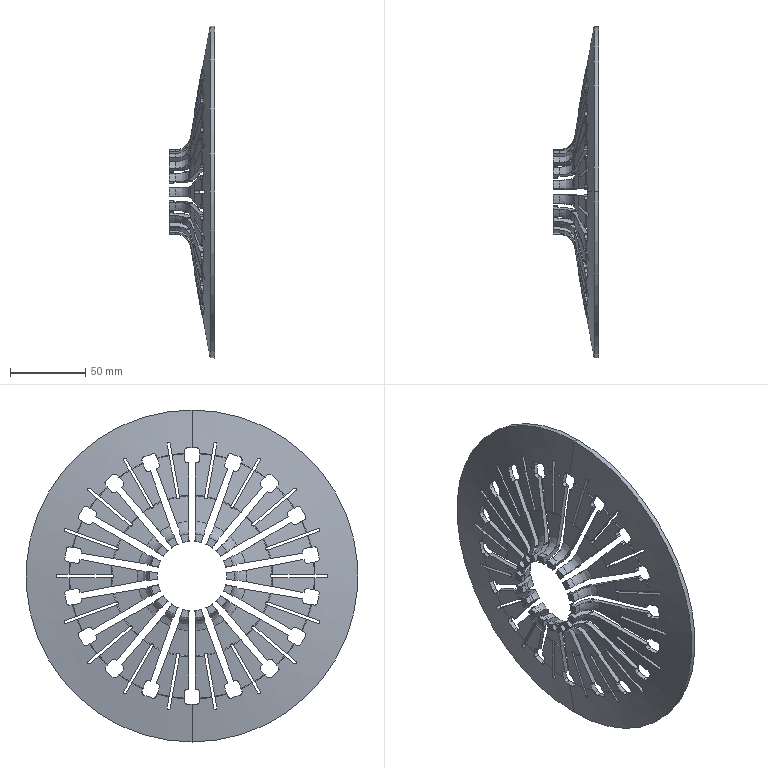Part | SolidWorks | features ICE 3, CirPattern 1, Revolution 1 | 1 solid | 848 faces | box 30 x 220 x 220 mm | volume 90672 mm3 | cylinder 286 | plane 270 | torus 180 | cone 112 | commonest cylinder face diameters 1 x90 4 x88 2 x52 46 x18 50 x18 56 x18